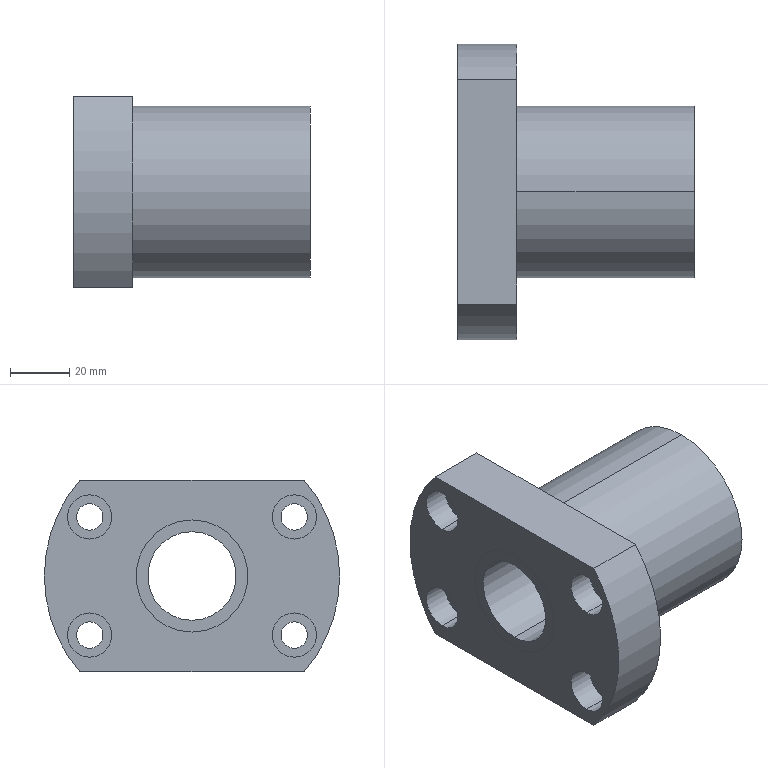Part | SolidWorks | features ICE 3, HoleWzd 1, Revolution 1 | 3 solids | 43 faces | box 80 x 100 x 65 mm | volume 212969 mm3 | cylinder 30 | plane 13 | commonest cylinder face diameters 9 x8 15 x8 38 x6 30 x4 58 x2 100 x2
STEP:
#1=CARTESIAN_POINT('',(9.,34.641,12.5));
#2=VERTEX_POINT('',#1);
#3=CARTESIAN_POINT('',(9.,34.641,27.5));
#4=VERTEX_POINT('',#3);
#5=CARTESIAN_POINT('',(9.,34.641,20.));
#6=DIRECTION('',(-1.,0.,0.));
#7=DIRECTION('',(0.,0.,1.));
#8=AXIS2_PLACEMENT_3D('',#5,#6,#7);
#9=CIRCLE('',#8,7.5);
#10=EDGE_CURVE('',#2,#4,#9,.T.);
#11=ORIENTED_EDGE('',*,*,#10,.F.);
#12=CARTESIAN_POINT('',(0.,34.641,12.5));
#13=VERTEX_POINT('',#12);
#14=CARTESIAN_POINT('',(0.,34.641,12.5));
#15=DIRECTION('',(-1.,0.,0.));
#16=VECTOR('',#15,1000.);
#17=LINE('',#14,#16);
#18=EDGE_CURVE('',#2,#13,#17,.T.);
#19=ORIENTED_EDGE('',*,*,#18,.T.);
#20=CARTESIAN_POINT('',(0.,34.641,27.5));
#21=VERTEX_POINT('',#20);
#22=CARTESIAN_POINT('',(0.,34.641,20.));
#23=DIRECTION('',(-1.,0.,0.));
#24=DIRECTION('',(0.,0.,1.));
#25=AXIS2_PLACEMENT_3D('',#22,#23,#24);
#26=CIRCLE('',#25,7.5);
#27=EDGE_CURVE('',#13,#21,#26,.T.);
#28=ORIENTED_EDGE('',*,*,#27,.T.);
#29=CARTESIAN_POINT('',(0.,34.641,27.5));
#30=DIRECTION('',(-1.,0.,0.));
#31=VECTOR('',#30,1000.);
#32=LINE('',#29,#31);
#33=EDGE_CURVE('',#4,#21,#32,.T.);
#34=ORIENTED_EDGE('',*,*,#33,.F.);
#35=EDGE_LOOP('',(#11,#19,#28,#34));
#36=FACE_OUTER_BOUND('',#35,.T.);
#37=CARTESIAN_POINT('',(0.,34.641,20.));
#38=DIRECTION('',(-1.,0.,0.));
#39=DIRECTION('',(0.,0.,1.));
#40=AXIS2_PLACEMENT_3D('',#37,#38,#39);
#41=CYLINDRICAL_SURFACE('',#40,7.5);
#42=ADVANCED_FACE('',(#36),#41,.F.);
#43=CARTESIAN_POINT('',(20.,34.641,15.5));
#44=VERTEX_POINT('',#43);
#45=CARTESIAN_POINT('',(20.,34.641,24.5));
#46=VERTEX_POINT('',#45);
#47=CARTESIAN_POINT('',(20.,34.641,20.));
#48=DIRECTION('',(-1.,0.,0.));
#49=DIRECTION('',(0.,0.,1.));
#50=AXIS2_PLACEMENT_3D('',#47,#48,#49);
#51=CIRCLE('',#50,4.5);
#52=EDGE_CURVE('',#44,#46,#51,.T.);
#53=ORIENTED_EDGE('',*,*,#52,.F.);
#54=CARTESIAN_POINT('',(9.,34.641,15.5));
#55=VERTEX_POINT('',#54);
#56=CARTESIAN_POINT('',(0.,34.641,15.5));
#57=DIRECTION('',(-1.,0.,0.));
#58=VECTOR('',#57,1000.);
#59=LINE('',#56,#58);
#60=EDGE_CURVE('',#44,#55,#59,.T.);
#61=ORIENTED_EDGE('',*,*,#60,.T.);
#62=CARTESIAN_POINT('',(9.,34.641,24.5));
#63=VERTEX_POINT('',#62);
#64=CARTESIAN_POINT('',(9.,34.641,20.));
#65=DIRECTION('',(-1.,0.,0.));
#66=DIRECTION('',(0.,0.,1.));
#67=AXIS2_PLACEMENT_3D('',#64,#65,#66);
#68=CIRCLE('',#67,4.5);
#69=EDGE_CURVE('',#55,#63,#68,.T.);
#70=ORIENTED_EDGE('',*,*,#69,.T.);
#71=CARTESIAN_POINT('',(0.,34.641,24.5));
#72=DIRECTION('',(-1.,0.,0.));
#73=VECTOR('',#72,1000.);
#74=LINE('',#71,#73);
#75=EDGE_CURVE('',#46,#63,#74,.T.);
#76=ORIENTED_EDGE('',*,*,#75,.F.);
#77=EDGE_LOOP('',(#53,#61,#70,#76));
#78=FACE_OUTER_BOUND('',#77,.T.);
#79=CARTESIAN_POINT('',(0.,34.641,20.));
#80=DIRECTION('',(-1.,0.,0.));
#81=DIRECTION('',(0.,0.,1.));
#82=AXIS2_PLACEMENT_3D('',#79,#80,#81);
#83=CYLINDRICAL_SURFACE('',#82,4.5);
#84=ADVANCED_FACE('',(#78),#83,.F.);
#85=CARTESIAN_POINT('',(9.,34.641,-27.5));
#86=VERTEX_POINT('',#85);
#87=CARTESIAN_POINT('',(9.,34.641,-12.5));
#88=VERTEX_POINT('',#87);
#89=CARTESIAN_POINT('',(9.,34.641,-20.));
#90=DIRECTION('',(-1.,0.,0.));
#91=DIRECTION('',(0.,0.,1.));
#92=AXIS2_PLACEMENT_3D('',#89,#90,#91);
#93=CIRCLE('',#92,7.5);
#94=EDGE_CURVE('',#86,#88,#93,.T.);
#95=ORIENTED_EDGE('',*,*,#94,.F.);
#96=CARTESIAN_POINT('',(0.,34.641,-27.5));
#97=VERTEX_POINT('',#96);
#98=CARTESIAN_POINT('',(0.,34.641,-27.5));
#99=DIRECTION('',(-1.,0.,0.));
#100=VECTOR('',#99,1000.);
#101=LINE('',#98,#100);
#102=EDGE_CURVE('',#86,#97,#101,.T.);
#103=ORIENTED_EDGE('',*,*,#102,.T.);
#104=CARTESIAN_POINT('',(0.,34.641,-12.5));
#105=VERTEX_POINT('',#104);
#106=CARTESIAN_POINT('',(0.,34.641,-20.));
#107=DIRECTION('',(-1.,0.,0.));
#108=DIRECTION('',(0.,0.,1.));
#109=AXIS2_PLACEMENT_3D('',#106,#107,#108);
#110=CIRCLE('',#109,7.5);
#111=EDGE_CURVE('',#97,#105,#110,.T.);
#112=ORIENTED_EDGE('',*,*,#111,.T.);
#113=CARTESIAN_POINT('',(0.,34.641,-12.5));
#114=DIRECTION('',(-1.,0.,0.));
#115=VECTOR('',#114,1000.);
#116=LINE('',#113,#115);
#117=EDGE_CURVE('',#88,#105,#116,.T.);
#118=ORIENTED_EDGE('',*,*,#117,.F.);
#119=EDGE_LOOP('',(#95,#103,#112,#118));
#120=FACE_OUTER_BOUND('',#119,.T.);
#121=CARTESIAN_POINT('',(0.,34.641,-20.));
#122=DIRECTION('',(-1.,0.,0.));
#123=DIRECTION('',(0.,0.,1.));
#124=AXIS2_PLACEMENT_3D('',#121,#122,#123);
#125=CYLINDRICAL_SURFACE('',#124,7.5);
#126=ADVANCED_FACE('',(#120),#125,.F.);
#127=CARTESIAN_POINT('',(20.,34.641,-24.5));
#128=VERTEX_POINT('',#127);
#129=CARTESIAN_POINT('',(20.,34.641,-15.5));
#130=VERTEX_POINT('',#129);
#131=CARTESIAN_POINT('',(20.,34.641,-20.));
#132=DIRECTION('',(-1.,0.,0.));
#133=DIRECTION('',(0.,0.,1.));
#134=AXIS2_PLACEMENT_3D('',#131,#132,#133);
#135=CIRCLE('',#134,4.5);
#136=EDGE_CURVE('',#128,#130,#135,.T.);
#137=ORIENTED_EDGE('',*,*,#136,.F.);
#138=CARTESIAN_POINT('',(9.,34.641,-24.5));
#139=VERTEX_POINT('',#138);
#140=CARTESIAN_POINT('',(0.,34.641,-24.5));
#141=DIRECTION('',(-1.,0.,0.));
#142=VECTOR('',#141,1000.);
#143=LINE('',#140,#142);
#144=EDGE_CURVE('',#128,#139,#143,.T.);
#145=ORIENTED_EDGE('',*,*,#144,.T.);
#146=CARTESIAN_POINT('',(9.,34.641,-15.5));
#147=VERTEX_POINT('',#146);
#148=CARTESIAN_POINT('',(9.,34.641,-20.));
#149=DIRECTION('',(-1.,0.,0.));
#150=DIRECTION('',(0.,0.,1.));
#151=AXIS2_PLACEMENT_3D('',#148,#149,#150);
#152=CIRCLE('',#151,4.5);
#153=EDGE_CURVE('',#139,#147,#152,.T.);
#154=ORIENTED_EDGE('',*,*,#153,.T.);
#155=CARTESIAN_POINT('',(0.,34.641,-15.5));
#156=DIRECTION('',(-1.,0.,0.));
#157=VECTOR('',#156,1000.);
#158=LINE('',#155,#157);
#159=EDGE_CURVE('',#130,#147,#158,.T.);
#160=ORIENTED_EDGE('',*,*,#159,.F.);
#161=EDGE_LOOP('',(#137,#145,#154,#160));
#162=FACE_OUTER_BOUND('',#161,.T.);
#163=CARTESIAN_POINT('',(0.,34.641,-20.));
#164=DIRECTION('',(-1.,0.,0.));
#165=DIRECTION('',(0.,0.,1.));
#166=AXIS2_PLACEMENT_3D('',#163,#164,#165);
#167=CYLINDRICAL_SURFACE('',#166,4.5);
#168=ADVANCED_FACE('',(#162),#167,.F.);
#169=CARTESIAN_POINT('',(9.,-34.641,-27.5));
#170=VERTEX_POINT('',#169);
#171=CARTESIAN_POINT('',(9.,-34.641,-12.5));
#172=VERTEX_POINT('',#171);
#173=CARTESIAN_POINT('',(9.,-34.641,-20.));
#174=DIRECTION('',(-1.,0.,0.));
#175=DIRECTION('',(0.,0.,1.));
#176=AXIS2_PLACEMENT_3D('',#173,#174,#175);
#177=CIRCLE('',#176,7.5);
#178=EDGE_CURVE('',#170,#172,#177,.T.);
#179=ORIENTED_EDGE('',*,*,#178,.F.);
#180=CARTESIAN_POINT('',(0.,-34.641,-27.5));
#181=VERTEX_POINT('',#180);
#182=CARTESIAN_POINT('',(0.,-34.641,-27.5));
#183=DIRECTION('',(-1.,0.,0.));
#184=VECTOR('',#183,1000.);
#185=LINE('',#182,#184);
#186=EDGE_CURVE('',#170,#181,#185,.T.);
#187=ORIENTED_EDGE('',*,*,#186,.T.);
#188=CARTESIAN_POINT('',(0.,-34.641,-12.5));
#189=VERTEX_POINT('',#188);
#190=CARTESIAN_POINT('',(0.,-34.641,-20.));
#191=DIRECTION('',(-1.,0.,0.));
#192=DIRECTION('',(0.,0.,1.));
#193=AXIS2_PLACEMENT_3D('',#190,#191,#192);
#194=CIRCLE('',#193,7.5);
#195=EDGE_CURVE('',#181,#189,#194,.T.);
#196=ORIENTED_EDGE('',*,*,#195,.T.);
#197=CARTESIAN_POINT('',(0.,-34.641,-12.5));
#198=DIRECTION('',(-1.,0.,0.));
#199=VECTOR('',#198,1000.);
#200=LINE('',#197,#199);
#201=EDGE_CURVE('',#172,#189,#200,.T.);
#202=ORIENTED_EDGE('',*,*,#201,.F.);
#203=EDGE_LOOP('',(#179,#187,#196,#202));
#204=FACE_OUTER_BOUND('',#203,.T.);
#205=CARTESIAN_POINT('',(0.,-34.641,-20.));
#206=DIRECTION('',(-1.,0.,0.));
#207=DIRECTION('',(0.,0.,1.));
#208=AXIS2_PLACEMENT_3D('',#205,#206,#207);
#209=CYLINDRICAL_SURFACE('',#208,7.5);
#210=ADVANCED_FACE('',(#204),#209,.F.);
#211=CARTESIAN_POINT('',(20.,-34.641,-24.5));
#212=VERTEX_POINT('',#211);
#213=CARTESIAN_POINT('',(20.,-34.641,-15.5));
#214=VERTEX_POINT('',#213);
#215=CARTESIAN_POINT('',(20.,-34.641,-20.));
#216=DIRECTION('',(-1.,0.,0.));
#217=DIRECTION('',(0.,0.,1.));
#218=AXIS2_PLACEMENT_3D('',#215,#216,#217);
#219=CIRCLE('',#218,4.5);
#220=EDGE_CURVE('',#212,#214,#219,.T.);
#221=ORIENTED_EDGE('',*,*,#220,.F.);
#222=CARTESIAN_POINT('',(9.,-34.641,-24.5));
#223=VERTEX_POINT('',#222);
#224=CARTESIAN_POINT('',(0.,-34.641,-24.5));
#225=DIRECTION('',(-1.,0.,0.));
#226=VECTOR('',#225,1000.);
#227=LINE('',#224,#226);
#228=EDGE_CURVE('',#212,#223,#227,.T.);
#229=ORIENTED_EDGE('',*,*,#228,.T.);
#230=CARTESIAN_POINT('',(9.,-34.641,-15.5));
#231=VERTEX_POINT('',#230);
#232=CARTESIAN_POINT('',(9.,-34.641,-20.));
#233=DIRECTION('',(-1.,0.,0.));
#234=DIRECTION('',(0.,0.,1.));
#235=AXIS2_PLACEMENT_3D('',#232,#233,#234);
#236=CIRCLE('',#235,4.5);
#237=EDGE_CURVE('',#223,#231,#236,.T.);
#238=ORIENTED_EDGE('',*,*,#237,.T.);
#239=CARTESIAN_POINT('',(0.,-34.641,-15.5));
#240=DIRECTION('',(-1.,0.,0.));
#241=VECTOR('',#240,1000.);
#242=LINE('',#239,#241);
#243=EDGE_CURVE('',#214,#231,#242,.T.);
#244=ORIENTED_EDGE('',*,*,#243,.F.);
#245=EDGE_LOOP('',(#221,#229,#238,#244));
#246=FACE_OUTER_BOUND('',#245,.T.);
#247=CARTESIAN_POINT('',(0.,-34.641,-20.));
#248=DIRECTION('',(-1.,0.,0.));
#249=DIRECTION('',(0.,0.,1.));
#250=AXIS2_PLACEMENT_3D('',#247,#248,#249);
#251=CYLINDRICAL_SURFACE('',#250,4.5);
#252=ADVANCED_FACE('',(#246),#251,.F.);
#253=CARTESIAN_POINT('',(9.,-34.641,12.5));
#254=VERTEX_POINT('',#253);
#255=CARTESIAN_POINT('',(9.,-34.641,27.5));
#256=VERTEX_POINT('',#255);
#257=CARTESIAN_POINT('',(9.,-34.641,20.));
#258=DIRECTION('',(-1.,0.,0.));
#259=DIRECTION('',(0.,0.,1.));
#260=AXIS2_PLACEMENT_3D('',#257,#258,#259);
#261=CIRCLE('',#260,7.5);
#262=EDGE_CURVE('',#254,#256,#261,.T.);
#263=ORIENTED_EDGE('',*,*,#262,.F.);
#264=CARTESIAN_POINT('',(0.,-34.641,12.5));
#265=VERTEX_POINT('',#264);
#266=CARTESIAN_POINT('',(0.,-34.641,12.5));
#267=DIRECTION('',(-1.,0.,0.));
#268=VECTOR('',#267,1000.);
#269=LINE('',#266,#268);
#270=EDGE_CURVE('',#254,#265,#269,.T.);
#271=ORIENTED_EDGE('',*,*,#270,.T.);
#272=CARTESIAN_POINT('',(0.,-34.641,27.5));
#273=VERTEX_POINT('',#272);
#274=CARTESIAN_POINT('',(0.,-34.641,20.));
#275=DIRECTION('',(-1.,0.,0.));
#276=DIRECTION('',(0.,0.,1.));
#277=AXIS2_PLACEMENT_3D('',#274,#275,#276);
#278=CIRCLE('',#277,7.5);
#279=EDGE_CURVE('',#265,#273,#278,.T.);
#280=ORIENTED_EDGE('',*,*,#279,.T.);
#281=CARTESIAN_POINT('',(0.,-34.641,27.5));
#282=DIRECTION('',(-1.,0.,0.));
#283=VECTOR('',#282,1000.);
#284=LINE('',#281,#283);
#285=EDGE_CURVE('',#256,#273,#284,.T.);
#286=ORIENTED_EDGE('',*,*,#285,.F.);
#287=EDGE_LOOP('',(#263,#271,#280,#286));
#288=FACE_OUTER_BOUND('',#287,.T.);
#289=CARTESIAN_POINT('',(0.,-34.641,20.));
#290=DIRECTION('',(-1.,0.,0.));
#291=DIRECTION('',(0.,0.,1.));
#292=AXIS2_PLACEMENT_3D('',#289,#290,#291);
#293=CYLINDRICAL_SURFACE('',#292,7.5);
#294=ADVANCED_FACE('',(#288),#293,.F.);
#295=CARTESIAN_POINT('',(20.,-34.641,15.5));
#296=VERTEX_POINT('',#295);
#297=CARTESIAN_POINT('',(20.,-34.641,24.5));
#298=VERTEX_POINT('',#297);
#299=CARTESIAN_POINT('',(20.,-34.641,20.));
#300=DIRECTION('',(-1.,0.,0.));
#301=DIRECTION('',(0.,0.,1.));
#302=AXIS2_PLACEMENT_3D('',#299,#300,#301);
#303=CIRCLE('',#302,4.5);
#304=EDGE_CURVE('',#296,#298,#303,.T.);
#305=ORIENTED_EDGE('',*,*,#304,.F.);
#306=CARTESIAN_POINT('',(9.,-34.641,15.5));
#307=VERTEX_POINT('',#306);
#308=CARTESIAN_POINT('',(0.,-34.641,15.5));
#309=DIRECTION('',(-1.,0.,0.));
#310=VECTOR('',#309,1000.);
#311=LINE('',#308,#310);
#312=EDGE_CURVE('',#296,#307,#311,.T.);
#313=ORIENTED_EDGE('',*,*,#312,.T.);
#314=CARTESIAN_POINT('',(9.,-34.641,24.5));
#315=VERTEX_POINT('',#314);
#316=CARTESIAN_POINT('',(9.,-34.641,20.));
#317=DIRECTION('',(-1.,0.,0.));
#318=DIRECTION('',(0.,0.,1.));
#319=AXIS2_PLACEMENT_3D('',#316,#317,#318);
#320=CIRCLE('',#319,4.5);
#321=EDGE_CURVE('',#307,#315,#320,.T.);
#322=ORIENTED_EDGE('',*,*,#321,.T.);
#323=CARTESIAN_POINT('',(0.,-34.641,24.5));
#324=DIRECTION('',(-1.,0.,0.));
#325=VECTOR('',#324,1000.);
#326=LINE('',#323,#325);
#327=EDGE_CURVE('',#298,#315,#326,.T.);
#328=ORIENTED_EDGE('',*,*,#327,.F.);
#329=EDGE_LOOP('',(#305,#313,#322,#328));
#330=FACE_OUTER_BOUND('',#329,.T.);
#331=CARTESIAN_POINT('',(0.,-34.641,20.));
#332=DIRECTION('',(-1.,0.,0.));
#333=DIRECTION('',(0.,0.,1.));
#334=AXIS2_PLACEMENT_3D('',#331,#332,#333);
#335=CYLINDRICAL_SURFACE('',#334,4.5);
#336=ADVANCED_FACE('',(#330),#335,.F.);
#337=CARTESIAN_POINT('',(80.,0.,-19.));
#338=VERTEX_POINT('',#337);
#339=CARTESIAN_POINT('',(80.,0.,19.));
#340=VERTEX_POINT('',#339);
#341=CARTESIAN_POINT('',(80.,0.,0.));
#342=DIRECTION('',(-1.,0.,0.));
#343=DIRECTION('',(0.,0.,1.));
#344=AXIS2_PLACEMENT_3D('',#341,#342,#343);
#345=CIRCLE('',#344,19.);
#346=EDGE_CURVE('',#338,#340,#345,.T.);
#347=ORIENTED_EDGE('',*,*,#346,.F.);
#348=CARTESIAN_POINT('',(0.,0.,-19.));
#349=VERTEX_POINT('',#348);
#350=CARTESIAN_POINT('',(0.,0.,-19.));
#351=DIRECTION('',(-1.,0.,0.));
#352=VECTOR('',#351,1000.);
#353=LINE('',#350,#352);
#354=EDGE_CURVE('',#338,#349,#353,.T.);
#355=ORIENTED_EDGE('',*,*,#354,.T.);
#356=CARTESIAN_POINT('',(0.,0.,19.));
#357=VERTEX_POINT('',#356);
#358=CARTESIAN_POINT('',(0.,0.,0.));
#359=DIRECTION('',(-1.,0.,0.));
#360=DIRECTION('',(0.,0.,1.));
#361=AXIS2_PLACEMENT_3D('',#358,#359,#360);
#362=CIRCLE('',#361,19.);
#363=EDGE_CURVE('',#349,#357,#362,.T.);
#364=ORIENTED_EDGE('',*,*,#363,.T.);
#365=CARTESIAN_POINT('',(0.,0.,19.));
#366=DIRECTION('',(-1.,0.,0.));
#367=VECTOR('',#366,1000.);
#368=LINE('',#365,#367);
#369=EDGE_CURVE('',#340,#357,#368,.T.);
#370=ORIENTED_EDGE('',*,*,#369,.F.);
#371=EDGE_LOOP('',(#347,#355,#364,#370));
#372=FACE_OUTER_BOUND('',#371,.T.);
#373=CARTESIAN_POINT('',(0.,0.,0.));
#374=DIRECTION('',(-1.,0.,0.));
#375=DIRECTION('',(0.,0.,1.));
#376=AXIS2_PLACEMENT_3D('',#373,#374,#375);
#377=CYLINDRICAL_SURFACE('',#376,19.);
#378=ADVANCED_FACE('',(#372),#377,.F.);
#379=CARTESIAN_POINT('',(80.,0.,29.));
#380=VERTEX_POINT('',#379);
#381=CARTESIAN_POINT('',(80.,0.,-29.));
#382=VERTEX_POINT('',#381);
#383=CARTESIAN_POINT('',(80.,0.,0.));
#384=DIRECTION('',(-1.,0.,0.));
#385=DIRECTION('',(0.,0.,1.));
#386=AXIS2_PLACEMENT_3D('',#383,#384,#385);
#387=CIRCLE('',#386,29.);
#388=EDGE_CURVE('',#380,#382,#387,.T.);
#389=ORIENTED_EDGE('',*,*,#388,.T.);
#390=CARTESIAN_POINT('',(20.,0.,-29.));
#391=VERTEX_POINT('',#390);
#392=CARTESIAN_POINT('',(0.,0.,-29.));
#393=DIRECTION('',(-1.,0.,0.));
#394=VECTOR('',#393,1000.);
#395=LINE('',#392,#394);
#396=EDGE_CURVE('',#382,#391,#395,.T.);
#397=ORIENTED_EDGE('',*,*,#396,.T.);
#398=CARTESIAN_POINT('',(20.,0.,29.));
#399=VERTEX_POINT('',#398);
#400=CARTESIAN_POINT('',(20.,0.,0.));
#401=DIRECTION('',(-1.,0.,0.));
#402=DIRECTION('',(0.,0.,1.));
#403=AXIS2_PLACEMENT_3D('',#400,#401,#402);
#404=CIRCLE('',#403,29.);
#405=EDGE_CURVE('',#399,#391,#404,.T.);
#406=ORIENTED_EDGE('',*,*,#405,.F.);
#407=CARTESIAN_POINT('',(0.,0.,29.));
#408=DIRECTION('',(-1.,0.,0.));
#409=VECTOR('',#408,1000.);
#410=LINE('',#407,#409);
#411=EDGE_CURVE('',#380,#399,#410,.T.);
#412=ORIENTED_EDGE('',*,*,#411,.F.);
#413=EDGE_LOOP('',(#389,#397,#406,#412));
#414=FACE_OUTER_BOUND('',#413,.T.);
#415=CARTESIAN_POINT('',(0.,0.,0.));
#416=DIRECTION('',(-1.,0.,0.));
#417=DIRECTION('',(0.,0.,1.));
#418=AXIS2_PLACEMENT_3D('',#415,#416,#417);
#419=CYLINDRICAL_SURFACE('',#418,29.);
#420=ADVANCED_FACE('',(#414),#419,.T.);
#421=CARTESIAN_POINT('',(20.,37.997,32.5));
#422=VERTEX_POINT('',#421);
#423=CARTESIAN_POINT('',(0.,37.997,32.5));
#424=VERTEX_POINT('',#423);
#425=CARTESIAN_POINT('',(0.,37.997,32.5));
#426=DIRECTION('',(-1.,0.,0.));
#427=VECTOR('',#426,1000.);
#428=LINE('',#425,#427);
#429=EDGE_CURVE('',#422,#424,#428,.T.);
#430=ORIENTED_EDGE('',*,*,#429,.F.);
#431=CARTESIAN_POINT('',(20.,37.997,-32.5));
#432=VERTEX_POINT('',#431);
#433=CARTESIAN_POINT('',(20.,0.,0.));
#434=DIRECTION('',(-1.,0.,0.));
#435=DIRECTION('',(0.,0.,1.));
#436=AXIS2_PLACEMENT_3D('',#433,#434,#435);
#437=CIRCLE('',#436,50.);
#438=EDGE_CURVE('',#422,#432,#437,.T.);
#439=ORIENTED_EDGE('',*,*,#438,.T.);
#440=CARTESIAN_POINT('',(0.,37.997,-32.5));
#441=VERTEX_POINT('',#440);
#442=CARTESIAN_POINT('',(0.,37.997,-32.5));
#443=DIRECTION('',(1.,0.,0.));
#444=VECTOR('',#443,1000.);
#445=LINE('',#442,#444);
#446=EDGE_CURVE('',#441,#432,#445,.T.);
#447=ORIENTED_EDGE('',*,*,#446,.F.);
#448=CARTESIAN_POINT('',(0.,0.,0.));
#449=DIRECTION('',(-1.,0.,0.));
#450=DIRECTION('',(0.,0.,1.));
#451=AXIS2_PLACEMENT_3D('',#448,#449,#450);
#452=CIRCLE('',#451,50.);
#453=EDGE_CURVE('',#424,#441,#452,.T.);
#454=ORIENTED_EDGE('',*,*,#453,.F.);
#455=EDGE_LOOP('',(#430,#439,#447,#454));
#456=FACE_OUTER_BOUND('',#455,.T.);
#457=CARTESIAN_POINT('',(0.,0.,0.));
#458=DIRECTION('',(-1.,0.,0.));
#459=DIRECTION('',(0.,0.,1.));
#460=AXIS2_PLACEMENT_3D('',#457,#458,#459);
#461=CYLINDRICAL_SURFACE('',#460,50.);
#462=ADVANCED_FACE('',(#456),#461,.T.);
#463=CARTESIAN_POINT('',(0.,-37.997,32.5));
#464=VERTEX_POINT('',#463);
#465=CARTESIAN_POINT('',(20.,-37.997,32.5));
#466=VERTEX_POINT('',#465);
#467=CARTESIAN_POINT('',(0.,-37.997,32.5));
#468=DIRECTION('',(1.,0.,0.));
#469=VECTOR('',#468,1000.);
#470=LINE('',#467,#469);
#471=EDGE_CURVE('',#464,#466,#470,.T.);
#472=ORIENTED_EDGE('',*,*,#471,.F.);
#473=CARTESIAN_POINT('',(0.,-37.997,-32.5));
#474=VERTEX_POINT('',#473);
#475=CARTESIAN_POINT('',(0.,0.,0.));
#476=DIRECTION('',(-1.,0.,0.));
#477=DIRECTION('',(0.,0.,1.));
#478=AXIS2_PLACEMENT_3D('',#475,#476,#477);
#479=CIRCLE('',#478,50.);
#480=EDGE_CURVE('',#474,#464,#479,.T.);
#481=ORIENTED_EDGE('',*,*,#480,.F.);
#482=CARTESIAN_POINT('',(20.,-37.997,-32.5));
#483=VERTEX_POINT('',#482);
#484=CARTESIAN_POINT('',(0.,-37.997,-32.5));
#485=DIRECTION('',(-1.,0.,0.));
#486=VECTOR('',#485,1000.);
#487=LINE('',#484,#486);
#488=EDGE_CURVE('',#483,#474,#487,.T.);
#489=ORIENTED_EDGE('',*,*,#488,.F.);
#490=CARTESIAN_POINT('',(20.,0.,0.));
#491=DIRECTION('',(-1.,0.,0.));
#492=DIRECTION('',(0.,0.,1.));
#493=AXIS2_PLACEMENT_3D('',#490,#491,#492);
#494=CIRCLE('',#493,50.);
#495=EDGE_CURVE('',#483,#466,#494,.T.);
#496=ORIENTED_EDGE('',*,*,#495,.T.);
#497=EDGE_LOOP('',(#472,#481,#489,#496));
#498=FACE_OUTER_BOUND('',#497,.T.);
#499=CARTESIAN_POINT('',(0.,0.,0.));
#500=DIRECTION('',(-1.,0.,0.));
#501=DIRECTION('',(0.,0.,1.));
#502=AXIS2_PLACEMENT_3D('',#499,#500,#501);
#503=CYLINDRICAL_SURFACE('',#502,50.);
#504=ADVANCED_FACE('',(#498),#503,.T.);
#505=CARTESIAN_POINT('',(20.,34.641,20.));
#506=DIRECTION('',(-1.,0.,0.));
#507=DIRECTION('',(0.,0.,1.));
#508=AXIS2_PLACEMENT_3D('',#505,#506,#507);
#509=CIRCLE('',#508,4.5);
#510=EDGE_CURVE('',#46,#44,#509,.T.);
#511=ORIENTED_EDGE('',*,*,#510,.T.);
#512=ORIENTED_EDGE('',*,*,#52,.T.);
#513=EDGE_LOOP('',(#511,#512));
#514=FACE_BOUND('',#513,.T.);
#515=CARTESIAN_POINT('',(20.,34.641,-20.));
#516=DIRECTION('',(-1.,0.,0.));
#517=DIRECTION('',(0.,0.,1.));
#518=AXIS2_PLACEMENT_3D('',#515,#516,#517);
#519=CIRCLE('',#518,4.5);
#520=EDGE_CURVE('',#130,#128,#519,.T.);
#521=ORIENTED_EDGE('',*,*,#520,.T.);
#522=ORIENTED_EDGE('',*,*,#136,.T.);
#523=EDGE_LOOP('',(#521,#522));
#524=FACE_BOUND('',#523,.T.);
#525=CARTESIAN_POINT('',(20.,-34.641,-20.));
#526=DIRECTION('',(-1.,0.,0.));
#527=DIRECTION('',(0.,0.,1.));
#528=AXIS2_PLACEMENT_3D('',#525,#526,#527);
#529=CIRCLE('',#528,4.5);
#530=EDGE_CURVE('',#214,#212,#529,.T.);
#531=ORIENTED_EDGE('',*,*,#530,.T.);
#532=ORIENTED_EDGE('',*,*,#220,.T.);
#533=EDGE_LOOP('',(#531,#532));
#534=FACE_BOUND('',#533,.T.);
#535=CARTESIAN_POINT('',(20.,-34.641,20.));
#536=DIRECTION('',(-1.,0.,0.));
#537=DIRECTION('',(0.,0.,1.));
#538=AXIS2_PLACEMENT_3D('',#535,#536,#537);
#539=CIRCLE('',#538,4.5);
#540=EDGE_CURVE('',#298,#296,#539,.T.);
#541=ORIENTED_EDGE('',*,*,#540,.T.);
#542=ORIENTED_EDGE('',*,*,#304,.T.);
#543=EDGE_LOOP('',(#541,#542));
#544=FACE_BOUND('',#543,.T.);
#545=ORIENTED_EDGE('',*,*,#405,.T.);
#546=CARTESIAN_POINT('',(20.,0.,0.));
#547=DIRECTION('',(-1.,0.,0.));
#548=DIRECTION('',(0.,0.,1.));
#549=AXIS2_PLACEMENT_3D('',#546,#547,#548);
#550=CIRCLE('',#549,29.);
#551=EDGE_CURVE('',#391,#399,#550,.T.);
#552=ORIENTED_EDGE('',*,*,#551,.T.);
#553=EDGE_LOOP('',(#545,#552));
#554=FACE_BOUND('',#553,.T.);
#555=CARTESIAN_POINT('',(20.,50.,32.5));
#556=DIRECTION('',(0.,1.,0.));
#557=VECTOR('',#556,1000.);
#558=LINE('',#555,#557);
#559=EDGE_CURVE('',#466,#422,#558,.T.);
#560=ORIENTED_EDGE('',*,*,#559,.F.);
#561=ORIENTED_EDGE('',*,*,#495,.F.);
#562=CARTESIAN_POINT('',(20.,50.,-32.5));
#563=DIRECTION('',(0.,-1.,0.));
#564=VECTOR('',#563,1000.);
#565=LINE('',#562,#564);
#566=EDGE_CURVE('',#432,#483,#565,.T.);
#567=ORIENTED_EDGE('',*,*,#566,.F.);
#568=ORIENTED_EDGE('',*,*,#438,.F.);
#569=EDGE_LOOP('',(#560,#561,#567,#568));
#570=FACE_OUTER_BOUND('',#569,.T.);
#571=CARTESIAN_POINT('',(20.,50.,0.));
#572=DIRECTION('',(-1.,0.,0.));
#573=DIRECTION('',(0.,0.,1.));
#574=AXIS2_PLACEMENT_3D('',#571,#572,#573);
#575=PLANE('',#574);
#576=ADVANCED_FACE('',(#514,#524,#534,#544,#554,#570),#575,.F.);
#577=CARTESIAN_POINT('',(0.,34.641,20.));
#578=DIRECTION('',(-1.,0.,0.));
#579=DIRECTION('',(0.,0.,1.));
#580=AXIS2_PLACEMENT_3D('',#577,#578,#579);
#581=CIRCLE('',#580,7.5);
#582=EDGE_CURVE('',#21,#13,#581,.T.);
#583=ORIENTED_EDGE('',*,*,#582,.F.);
#584=ORIENTED_EDGE('',*,*,#27,.F.);
#585=EDGE_LOOP('',(#583,#584));
#586=FACE_BOUND('',#585,.T.);
#587=CARTESIAN_POINT('',(0.,34.641,-20.));
#588=DIRECTION('',(-1.,0.,0.));
#589=DIRECTION('',(0.,0.,1.));
#590=AXIS2_PLACEMENT_3D('',#587,#588,#589);
#591=CIRCLE('',#590,7.5);
#592=EDGE_CURVE('',#105,#97,#591,.T.);
#593=ORIENTED_EDGE('',*,*,#592,.F.);
#594=ORIENTED_EDGE('',*,*,#111,.F.);
#595=EDGE_LOOP('',(#593,#594));
#596=FACE_BOUND('',#595,.T.);
#597=CARTESIAN_POINT('',(0.,-34.641,-20.));
#598=DIRECTION('',(-1.,0.,0.));
#599=DIRECTION('',(0.,0.,1.));
#600=AXIS2_PLACEMENT_3D('',#597,#598,#599);
#601=CIRCLE('',#600,7.5);
#602=EDGE_CURVE('',#189,#181,#601,.T.);
#603=ORIENTED_EDGE('',*,*,#602,.F.);
#604=ORIENTED_EDGE('',*,*,#195,.F.);
#605=EDGE_LOOP('',(#603,#604));
#606=FACE_BOUND('',#605,.T.);
#607=CARTESIAN_POINT('',(0.,-34.641,20.));
#608=DIRECTION('',(-1.,0.,0.));
#609=DIRECTION('',(0.,0.,1.));
#610=AXIS2_PLACEMENT_3D('',#607,#608,#609);
#611=CIRCLE('',#610,7.5);
#612=EDGE_CURVE('',#273,#265,#611,.T.);
#613=ORIENTED_EDGE('',*,*,#612,.F.);
#614=ORIENTED_EDGE('',*,*,#279,.F.);
#615=EDGE_LOOP('',(#613,#614));
#616=FACE_BOUND('',#615,.T.);
#617=CARTESIAN_POINT('',(0.,0.,0.));
#618=DIRECTION('',(-1.,0.,0.));
#619=DIRECTION('',(0.,0.,1.));
#620=AXIS2_PLACEMENT_3D('',#617,#618,#619);
#621=CIRCLE('',#620,19.);
#622=EDGE_CURVE('',#357,#349,#621,.T.);
#623=ORIENTED_EDGE('',*,*,#622,.F.);
#624=ORIENTED_EDGE('',*,*,#363,.F.);
#625=EDGE_LOOP('',(#623,#624));
#626=FACE_BOUND('',#625,.T.);
#627=CARTESIAN_POINT('',(0.,19.,32.5));
#628=DIRECTION('',(0.,-1.,0.));
#629=VECTOR('',#628,1000.);
#630=LINE('',#627,#629);
#631=EDGE_CURVE('',#424,#464,#630,.T.);
#632=ORIENTED_EDGE('',*,*,#631,.F.);
#633=ORIENTED_EDGE('',*,*,#453,.T.);
#634=CARTESIAN_POINT('',(0.,19.,-32.5));
#635=DIRECTION('',(0.,1.,0.));
#636=VECTOR('',#635,1000.);
#637=LINE('',#634,#636);
#638=EDGE_CURVE('',#474,#441,#637,.T.);
#639=ORIENTED_EDGE('',*,*,#638,.F.);
#640=ORIENTED_EDGE('',*,*,#480,.T.);
#641=EDGE_LOOP('',(#632,#633,#639,#640));
#642=FACE_OUTER_BOUND('',#641,.T.);
#643=CARTESIAN_POINT('',(0.,19.,0.));
#644=DIRECTION('',(1.,0.,0.));
#645=DIRECTION('',(0.,0.,-1.));
#646=AXIS2_PLACEMENT_3D('',#643,#644,#645);
#647=PLANE('',#646);
#648=ADVANCED_FACE('',(#586,#596,#606,#616,#626,#642),#647,.F.);
#649=ORIENTED_EDGE('',*,*,#396,.F.);
#650=CARTESIAN_POINT('',(80.,0.,0.));
#651=DIRECTION('',(-1.,0.,0.));
#652=DIRECTION('',(0.,0.,1.));
#653=AXIS2_PLACEMENT_3D('',#650,#651,#652);
#654=CIRCLE('',#653,29.);
#655=EDGE_CURVE('',#382,#380,#654,.T.);
#656=ORIENTED_EDGE('',*,*,#655,.T.);
#657=ORIENTED_EDGE('',*,*,#411,.T.);
#658=ORIENTED_EDGE('',*,*,#551,.F.);
#659=EDGE_LOOP('',(#649,#656,#657,#658));
#660=FACE_OUTER_BOUND('',#659,.T.);
#661=CARTESIAN_POINT('',(0.,0.,0.));
#662=DIRECTION('',(-1.,0.,0.));
#663=DIRECTION('',(0.,0.,1.));
#664=AXIS2_PLACEMENT_3D('',#661,#662,#663);
#665=CYLINDRICAL_SURFACE('',#664,29.);
#666=ADVANCED_FACE('',(#660),#665,.T.);
#667=ORIENTED_EDGE('',*,*,#388,.F.);
#668=ORIENTED_EDGE('',*,*,#655,.F.);
#669=EDGE_LOOP('',(#667,#668));
#670=FACE_OUTER_BOUND('',#669,.T.);
#671=CARTESIAN_POINT('',(80.,0.,0.));
#672=DIRECTION('',(-1.,0.,0.));
#673=DIRECTION('',(0.,0.,1.));
#674=AXIS2_PLACEMENT_3D('',#671,#672,#673);
#675=CIRCLE('',#674,19.);
#676=EDGE_CURVE('',#340,#338,#675,.T.);
#677=ORIENTED_EDGE('',*,*,#676,.T.);
#678=ORIENTED_EDGE('',*,*,#346,.T.);
#679=EDGE_LOOP('',(#677,#678));
#680=FACE_BOUND('',#679,.T.);
#681=CARTESIAN_POINT('',(80.,29.,0.));
#682=DIRECTION('',(-1.,0.,0.));
#683=DIRECTION('',(0.,0.,1.));
#684=AXIS2_PLACEMENT_3D('',#681,#682,#683);
#685=PLANE('',#684);
#686=ADVANCED_FACE('',(#670,#680),#685,.F.);
#687=ORIENTED_EDGE('',*,*,#354,.F.);
#688=ORIENTED_EDGE('',*,*,#676,.F.);
#689=ORIENTED_EDGE('',*,*,#369,.T.);
#690=ORIENTED_EDGE('',*,*,#622,.T.);
#691=EDGE_LOOP('',(#687,#688,#689,#690));
#692=FACE_OUTER_BOUND('',#691,.T.);
#693=CARTESIAN_POINT('',(0.,0.,0.));
#694=DIRECTION('',(-1.,0.,0.));
#695=DIRECTION('',(0.,0.,1.));
#696=AXIS2_PLACEMENT_3D('',#693,#694,#695);
#697=CYLINDRICAL_SURFACE('',#696,19.);
#698=ADVANCED_FACE('',(#692),#697,.F.);
#699=ORIENTED_EDGE('',*,*,#312,.F.);
#700=ORIENTED_EDGE('',*,*,#540,.F.);
#701=ORIENTED_EDGE('',*,*,#327,.T.);
#702=CARTESIAN_POINT('',(9.,-34.641,20.));
#703=DIRECTION('',(-1.,0.,0.));
#704=DIRECTION('',(0.,0.,1.));
#705=AXIS2_PLACEMENT_3D('',#702,#703,#704);
#706=CIRCLE('',#705,4.5);
#707=EDGE_CURVE('',#315,#307,#706,.T.);
#708=ORIENTED_EDGE('',*,*,#707,.T.);
#709=EDGE_LOOP('',(#699,#700,#701,#708));
#710=FACE_OUTER_BOUND('',#709,.T.);
#711=CARTESIAN_POINT('',(0.,-34.641,20.));
#712=DIRECTION('',(-1.,0.,0.));
#713=DIRECTION('',(0.,0.,1.));
#714=AXIS2_PLACEMENT_3D('',#711,#712,#713);
#715=CYLINDRICAL_SURFACE('',#714,4.5);
#716=ADVANCED_FACE('',(#710),#715,.F.);
#717=ORIENTED_EDGE('',*,*,#707,.F.);
#718=ORIENTED_EDGE('',*,*,#321,.F.);
#719=EDGE_LOOP('',(#717,#718));
#720=FACE_BOUND('',#719,.T.);
#721=CARTESIAN_POINT('',(9.,-34.641,20.));
#722=DIRECTION('',(-1.,0.,0.));
#723=DIRECTION('',(0.,0.,1.));
#724=AXIS2_PLACEMENT_3D('',#721,#722,#723);
#725=CIRCLE('',#724,7.5);
#726=EDGE_CURVE('',#256,#254,#725,.T.);
#727=ORIENTED_EDGE('',*,*,#726,.T.);
#728=ORIENTED_EDGE('',*,*,#262,.T.);
#729=EDGE_LOOP('',(#727,#728));
#730=FACE_OUTER_BOUND('',#729,.T.);
#731=CARTESIAN_POINT('',(9.,-30.141,20.));
#732=DIRECTION('',(1.,0.,0.));
#733=DIRECTION('',(0.,0.,-1.));
#734=AXIS2_PLACEMENT_3D('',#731,#732,#733);
#735=PLANE('',#734);
#736=ADVANCED_FACE('',(#720,#730),#735,.F.);
#737=ORIENTED_EDGE('',*,*,#270,.F.);
#738=ORIENTED_EDGE('',*,*,#726,.F.);
#739=ORIENTED_EDGE('',*,*,#285,.T.);
#740=ORIENTED_EDGE('',*,*,#612,.T.);
#741=EDGE_LOOP('',(#737,#738,#739,#740));
#742=FACE_OUTER_BOUND('',#741,.T.);
#743=CARTESIAN_POINT('',(0.,-34.641,20.));
#744=DIRECTION('',(-1.,0.,0.));
#745=DIRECTION('',(0.,0.,1.));
#746=AXIS2_PLACEMENT_3D('',#743,#744,#745);
#747=CYLINDRICAL_SURFACE('',#746,7.5);
#748=ADVANCED_FACE('',(#742),#747,.F.);
#749=ORIENTED_EDGE('',*,*,#228,.F.);
#750=ORIENTED_EDGE('',*,*,#530,.F.);
#751=ORIENTED_EDGE('',*,*,#243,.T.);
#752=CARTESIAN_POINT('',(9.,-34.641,-20.));
#753=DIRECTION('',(-1.,0.,0.));
#754=DIRECTION('',(0.,0.,1.));
#755=AXIS2_PLACEMENT_3D('',#752,#753,#754);
#756=CIRCLE('',#755,4.5);
#757=EDGE_CURVE('',#231,#223,#756,.T.);
#758=ORIENTED_EDGE('',*,*,#757,.T.);
#759=EDGE_LOOP('',(#749,#750,#751,#758));
#760=FACE_OUTER_BOUND('',#759,.T.);
#761=CARTESIAN_POINT('',(0.,-34.641,-20.));
#762=DIRECTION('',(-1.,0.,0.));
#763=DIRECTION('',(0.,0.,1.));
#764=AXIS2_PLACEMENT_3D('',#761,#762,#763);
#765=CYLINDRICAL_SURFACE('',#764,4.5);
#766=ADVANCED_FACE('',(#760),#765,.F.);
#767=ORIENTED_EDGE('',*,*,#757,.F.);
#768=ORIENTED_EDGE('',*,*,#237,.F.);
#769=EDGE_LOOP('',(#767,#768));
#770=FACE_BOUND('',#769,.T.);
#771=CARTESIAN_POINT('',(9.,-34.641,-20.));
#772=DIRECTION('',(-1.,0.,0.));
#773=DIRECTION('',(0.,0.,1.));
#774=AXIS2_PLACEMENT_3D('',#771,#772,#773);
#775=CIRCLE('',#774,7.5);
#776=EDGE_CURVE('',#172,#170,#775,.T.);
#777=ORIENTED_EDGE('',*,*,#776,.T.);
#778=ORIENTED_EDGE('',*,*,#178,.T.);
#779=EDGE_LOOP('',(#777,#778));
#780=FACE_OUTER_BOUND('',#779,.T.);
#781=CARTESIAN_POINT('',(9.,-30.141,-20.));
#782=DIRECTION('',(1.,0.,0.));
#783=DIRECTION('',(0.,0.,-1.));
#784=AXIS2_PLACEMENT_3D('',#781,#782,#783);
#785=PLANE('',#784);
#786=ADVANCED_FACE('',(#770,#780),#785,.F.);
#787=ORIENTED_EDGE('',*,*,#186,.F.);
#788=ORIENTED_EDGE('',*,*,#776,.F.);
#789=ORIENTED_EDGE('',*,*,#201,.T.);
#790=ORIENTED_EDGE('',*,*,#602,.T.);
#791=EDGE_LOOP('',(#787,#788,#789,#790));
#792=FACE_OUTER_BOUND('',#791,.T.);
#793=CARTESIAN_POINT('',(0.,-34.641,-20.));
#794=DIRECTION('',(-1.,0.,0.));
#795=DIRECTION('',(0.,0.,1.));
#796=AXIS2_PLACEMENT_3D('',#793,#794,#795);
#797=CYLINDRICAL_SURFACE('',#796,7.5);
#798=ADVANCED_FACE('',(#792),#797,.F.);
#799=ORIENTED_EDGE('',*,*,#144,.F.);
#800=ORIENTED_EDGE('',*,*,#520,.F.);
#801=ORIENTED_EDGE('',*,*,#159,.T.);
#802=CARTESIAN_POINT('',(9.,34.641,-20.));
#803=DIRECTION('',(-1.,0.,0.));
#804=DIRECTION('',(0.,0.,1.));
#805=AXIS2_PLACEMENT_3D('',#802,#803,#804);
#806=CIRCLE('',#805,4.5);
#807=EDGE_CURVE('',#147,#139,#806,.T.);
#808=ORIENTED_EDGE('',*,*,#807,.T.);
#809=EDGE_LOOP('',(#799,#800,#801,#808));
#810=FACE_OUTER_BOUND('',#809,.T.);
#811=CARTESIAN_POINT('',(0.,34.641,-20.));
#812=DIRECTION('',(-1.,0.,0.));
#813=DIRECTION('',(0.,0.,1.));
#814=AXIS2_PLACEMENT_3D('',#811,#812,#813);
#815=CYLINDRICAL_SURFACE('',#814,4.5);
#816=ADVANCED_FACE('',(#810),#815,.F.);
#817=ORIENTED_EDGE('',*,*,#807,.F.);
#818=ORIENTED_EDGE('',*,*,#153,.F.);
#819=EDGE_LOOP('',(#817,#818));
#820=FACE_BOUND('',#819,.T.);
#821=CARTESIAN_POINT('',(9.,34.641,-20.));
#822=DIRECTION('',(-1.,0.,0.));
#823=DIRECTION('',(0.,0.,1.));
#824=AXIS2_PLACEMENT_3D('',#821,#822,#823);
#825=CIRCLE('',#824,7.5);
#826=EDGE_CURVE('',#88,#86,#825,.T.);
#827=ORIENTED_EDGE('',*,*,#826,.T.);
#828=ORIENTED_EDGE('',*,*,#94,.T.);
#829=EDGE_LOOP('',(#827,#828));
#830=FACE_OUTER_BOUND('',#829,.T.);
#831=CARTESIAN_POINT('',(9.,39.141,-20.));
#832=DIRECTION('',(1.,0.,0.));
#833=DIRECTION('',(0.,0.,-1.));
#834=AXIS2_PLACEMENT_3D('',#831,#832,#833);
#835=PLANE('',#834);
#836=ADVANCED_FACE('',(#820,#830),#835,.F.);
#837=ORIENTED_EDGE('',*,*,#102,.F.);
#838=ORIENTED_EDGE('',*,*,#826,.F.);
#839=ORIENTED_EDGE('',*,*,#117,.T.);
#840=ORIENTED_EDGE('',*,*,#592,.T.);
#841=EDGE_LOOP('',(#837,#838,#839,#840));
#842=FACE_OUTER_BOUND('',#841,.T.);
#843=CARTESIAN_POINT('',(0.,34.641,-20.));
#844=DIRECTION('',(-1.,0.,0.));
#845=DIRECTION('',(0.,0.,1.));
#846=AXIS2_PLACEMENT_3D('',#843,#844,#845);
#847=CYLINDRICAL_SURFACE('',#846,7.5);
#848=ADVANCED_FACE('',(#842),#847,.F.);
#849=ORIENTED_EDGE('',*,*,#60,.F.);
#850=ORIENTED_EDGE('',*,*,#510,.F.);
#851=ORIENTED_EDGE('',*,*,#75,.T.);
#852=CARTESIAN_POINT('',(9.,34.641,20.));
#853=DIRECTION('',(-1.,0.,0.));
#854=DIRECTION('',(0.,0.,1.));
#855=AXIS2_PLACEMENT_3D('',#852,#853,#854);
#856=CIRCLE('',#855,4.5);
#857=EDGE_CURVE('',#63,#55,#856,.T.);
#858=ORIENTED_EDGE('',*,*,#857,.T.);
#859=EDGE_LOOP('',(#849,#850,#851,#858));
#860=FACE_OUTER_BOUND('',#859,.T.);
#861=CARTESIAN_POINT('',(0.,34.641,20.));
#862=DIRECTION('',(-1.,0.,0.));
#863=DIRECTION('',(0.,0.,1.));
#864=AXIS2_PLACEMENT_3D('',#861,#862,#863);
#865=CYLINDRICAL_SURFACE('',#864,4.5);
#866=ADVANCED_FACE('',(#860),#865,.F.);
#867=ORIENTED_EDGE('',*,*,#857,.F.);
#868=ORIENTED_EDGE('',*,*,#69,.F.);
#869=EDGE_LOOP('',(#867,#868));
#870=FACE_BOUND('',#869,.T.);
#871=CARTESIAN_POINT('',(9.,34.641,20.));
#872=DIRECTION('',(-1.,0.,0.));
#873=DIRECTION('',(0.,0.,1.));
#874=AXIS2_PLACEMENT_3D('',#871,#872,#873);
#875=CIRCLE('',#874,7.5);
#876=EDGE_CURVE('',#4,#2,#875,.T.);
#877=ORIENTED_EDGE('',*,*,#876,.T.);
#878=ORIENTED_EDGE('',*,*,#10,.T.);
#879=EDGE_LOOP('',(#877,#878));
#880=FACE_OUTER_BOUND('',#879,.T.);
#881=CARTESIAN_POINT('',(9.,39.141,20.));
#882=DIRECTION('',(1.,0.,0.));
#883=DIRECTION('',(0.,0.,-1.));
#884=AXIS2_PLACEMENT_3D('',#881,#882,#883);
#885=PLANE('',#884);
#886=ADVANCED_FACE('',(#870,#880),#885,.F.);
#887=ORIENTED_EDGE('',*,*,#18,.F.);
#888=ORIENTED_EDGE('',*,*,#876,.F.);
#889=ORIENTED_EDGE('',*,*,#33,.T.);
#890=ORIENTED_EDGE('',*,*,#582,.T.);
#891=EDGE_LOOP('',(#887,#888,#889,#890));
#892=FACE_OUTER_BOUND('',#891,.T.);
#893=CARTESIAN_POINT('',(0.,34.641,20.));
#894=DIRECTION('',(-1.,0.,0.));
#895=DIRECTION('',(0.,0.,1.));
#896=AXIS2_PLACEMENT_3D('',#893,#894,#895);
#897=CYLINDRICAL_SURFACE('',#896,7.5);
#898=ADVANCED_FACE('',(#892),#897,.F.);
#899=ORIENTED_EDGE('',*,*,#488,.T.);
#900=ORIENTED_EDGE('',*,*,#638,.T.);
#901=ORIENTED_EDGE('',*,*,#446,.T.);
#902=ORIENTED_EDGE('',*,*,#566,.T.);
#903=EDGE_LOOP('',(#899,#900,#901,#902));
#904=FACE_OUTER_BOUND('',#903,.T.);
#905=CARTESIAN_POINT('',(80.,-55.,-32.5));
#906=DIRECTION('',(0.,0.,-1.));
#907=DIRECTION('',(-1.,0.,0.));
#908=AXIS2_PLACEMENT_3D('',#905,#906,#907);
#909=PLANE('',#908);
#910=ADVANCED_FACE('',(#904),#909,.T.);
#911=ORIENTED_EDGE('',*,*,#429,.T.);
#912=ORIENTED_EDGE('',*,*,#631,.T.);
#913=ORIENTED_EDGE('',*,*,#471,.T.);
#914=ORIENTED_EDGE('',*,*,#559,.T.);
#915=EDGE_LOOP('',(#911,#912,#913,#914));
#916=FACE_OUTER_BOUND('',#915,.T.);
#917=CARTESIAN_POINT('',(80.,-55.,32.5));
#918=DIRECTION('',(0.,0.,1.));
#919=DIRECTION('',(1.,0.,0.));
#920=AXIS2_PLACEMENT_3D('',#917,#918,#919);
#921=PLANE('',#920);
#922=ADVANCED_FACE('',(#916),#921,.T.);
#923=CLOSED_SHELL('',(#42,#84,#126,#168,#210,#252,#294,#336,#378,#420,#462,#504,#576,#648,#666,#686,#698,#716,#736,#748,#766,#786,#798,#816,#836,#848,#866,#886,#898,#910,#922));
#924=MANIFOLD_SOLID_BREP('',#923);
#925=CARTESIAN_POINT('',(40.,0.,15.));
#926=VERTEX_POINT('',#925);
#927=CARTESIAN_POINT('',(40.,0.,-15.));
#928=VERTEX_POINT('',#927);
#929=CARTESIAN_POINT('',(40.,0.,0.));
#930=DIRECTION('',(1.,0.,0.));
#931=DIRECTION('',(0.,0.,-1.));
#932=AXIS2_PLACEMENT_3D('',#929,#930,#931);
#933=CIRCLE('',#932,15.);
#934=EDGE_CURVE('',#926,#928,#933,.T.);
#935=ORIENTED_EDGE('',*,*,#934,.F.);
#936=CARTESIAN_POINT('',(80.,0.,15.));
#937=VERTEX_POINT('',#936);
#938=CARTESIAN_POINT('',(40.,0.,15.));
#939=DIRECTION('',(1.,0.,0.));
#940=VECTOR('',#939,1000.);
#941=LINE('',#938,#940);
#942=EDGE_CURVE('',#926,#937,#941,.T.);
#943=ORIENTED_EDGE('',*,*,#942,.T.);
#944=CARTESIAN_POINT('',(80.,0.,-15.));
#945=VERTEX_POINT('',#944);
#946=CARTESIAN_POINT('',(80.,0.,0.));
#947=DIRECTION('',(1.,0.,0.));
#948=DIRECTION('',(0.,0.,-1.));
#949=AXIS2_PLACEMENT_3D('',#946,#947,#948);
#950=CIRCLE('',#949,15.);
#951=EDGE_CURVE('',#937,#945,#950,.T.);
#952=ORIENTED_EDGE('',*,*,#951,.T.);
#953=CARTESIAN_POINT('',(40.,0.,-15.));
#954=DIRECTION('',(1.,0.,0.));
#955=VECTOR('',#954,1000.);
#956=LINE('',#953,#955);
#957=EDGE_CURVE('',#928,#945,#956,.T.);
#958=ORIENTED_EDGE('',*,*,#957,.F.);
#959=EDGE_LOOP('',(#935,#943,#952,#958));
#960=FACE_OUTER_BOUND('',#959,.T.);
#961=CARTESIAN_POINT('',(40.,0.,0.));
#962=DIRECTION('',(1.,0.,0.));
#963=DIRECTION('',(0.,0.,-1.));
#964=AXIS2_PLACEMENT_3D('',#961,#962,#963);
#965=CYLINDRICAL_SURFACE('',#964,15.);
#966=ADVANCED_FACE('',(#960),#965,.F.);
#967=CARTESIAN_POINT('',(40.,0.,-19.));
#968=VERTEX_POINT('',#967);
#969=CARTESIAN_POINT('',(40.,0.,19.));
#970=VERTEX_POINT('',#969);
#971=CARTESIAN_POINT('',(40.,0.,0.));
#972=DIRECTION('',(1.,0.,0.));
#973=DIRECTION('',(0.,0.,-1.));
#974=AXIS2_PLACEMENT_3D('',#971,#972,#973);
#975=CIRCLE('',#974,19.);
#976=EDGE_CURVE('',#968,#970,#975,.T.);
#977=ORIENTED_EDGE('',*,*,#976,.T.);
#978=CARTESIAN_POINT('',(80.,0.,19.));
#979=VERTEX_POINT('',#978);
#980=CARTESIAN_POINT('',(40.,0.,19.));
#981=DIRECTION('',(1.,0.,0.));
#982=VECTOR('',#981,1000.);
#983=LINE('',#980,#982);
#984=EDGE_CURVE('',#970,#979,#983,.T.);
#985=ORIENTED_EDGE('',*,*,#984,.T.);
#986=CARTESIAN_POINT('',(80.,0.,-19.));
#987=VERTEX_POINT('',#986);
#988=CARTESIAN_POINT('',(80.,0.,0.));
#989=DIRECTION('',(1.,0.,0.));
#990=DIRECTION('',(0.,0.,-1.));
#991=AXIS2_PLACEMENT_3D('',#988,#989,#990);
#992=CIRCLE('',#991,19.);
#993=EDGE_CURVE('',#987,#979,#992,.T.);
#994=ORIENTED_EDGE('',*,*,#993,.F.);
#995=CARTESIAN_POINT('',(40.,0.,-19.));
#996=DIRECTION('',(1.,0.,0.));
#997=VECTOR('',#996,1000.);
#998=LINE('',#995,#997);
#999=EDGE_CURVE('',#968,#987,#998,.T.);
#1000=ORIENTED_EDGE('',*,*,#999,.F.);
#1001=EDGE_LOOP('',(#977,#985,#994,#1000));
#1002=FACE_OUTER_BOUND('',#1001,.T.);
#1003=CARTESIAN_POINT('',(40.,0.,0.));
#1004=DIRECTION('',(1.,0.,0.));
#1005=DIRECTION('',(0.,0.,-1.));
#1006=AXIS2_PLACEMENT_3D('',#1003,#1004,#1005);
#1007=CYLINDRICAL_SURFACE('',#1006,19.);
#1008=ADVANCED_FACE('',(#1002),#1007,.T.);
#1009=ORIENTED_EDGE('',*,*,#984,.F.);
#1010=CARTESIAN_POINT('',(40.,0.,0.));
#1011=DIRECTION('',(1.,0.,0.));
#1012=DIRECTION('',(0.,0.,-1.));
#1013=AXIS2_PLACEMENT_3D('',#1010,#1011,#1012);
#1014=CIRCLE('',#1013,19.);
#1015=EDGE_CURVE('',#970,#968,#1014,.T.);
#1016=ORIENTED_EDGE('',*,*,#1015,.T.);
#1017=ORIENTED_EDGE('',*,*,#999,.T.);
#1018=CARTESIAN_POINT('',(80.,0.,0.));
#1019=DIRECTION('',(1.,0.,0.));
#1020=DIRECTION('',(0.,0.,-1.));
#1021=AXIS2_PLACEMENT_3D('',#1018,#1019,#1020);
#1022=CIRCLE('',#1021,19.);
#1023=EDGE_CURVE('',#979,#987,#1022,.T.);
#1024=ORIENTED_EDGE('',*,*,#1023,.F.);
#1025=EDGE_LOOP('',(#1009,#1016,#1017,#1024));
#1026=FACE_OUTER_BOUND('',#1025,.T.);
#1027=CARTESIAN_POINT('',(40.,0.,0.));
#1028=DIRECTION('',(1.,0.,0.));
#1029=DIRECTION('',(0.,0.,-1.));
#1030=AXIS2_PLACEMENT_3D('',#1027,#1028,#1029);
#1031=CYLINDRICAL_SURFACE('',#1030,19.);
#1032=ADVANCED_FACE('',(#1026),#1031,.T.);
#1033=CARTESIAN_POINT('',(40.,0.,0.));
#1034=DIRECTION('',(1.,0.,0.));
#1035=DIRECTION('',(0.,0.,-1.));
#1036=AXIS2_PLACEMENT_3D('',#1033,#1034,#1035);
#1037=CIRCLE('',#1036,15.);
#1038=EDGE_CURVE('',#928,#926,#1037,.T.);
#1039=ORIENTED_EDGE('',*,*,#1038,.T.);
#1040=ORIENTED_EDGE('',*,*,#934,.T.);
#1041=EDGE_LOOP('',(#1039,#1040));
#1042=FACE_BOUND('',#1041,.T.);
#1043=ORIENTED_EDGE('',*,*,#976,.F.);
#1044=ORIENTED_EDGE('',*,*,#1015,.F.);
#1045=EDGE_LOOP('',(#1043,#1044));
#1046=FACE_OUTER_BOUND('',#1045,.T.);
#1047=CARTESIAN_POINT('',(40.,0.,0.));
#1048=DIRECTION('',(1.,0.,0.));
#1049=DIRECTION('',(0.,0.,-1.));
#1050=AXIS2_PLACEMENT_3D('',#1047,#1048,#1049);
#1051=PLANE('',#1050);
#1052=ADVANCED_FACE('',(#1042,#1046),#1051,.F.);
#1053=CARTESIAN_POINT('',(80.,0.,0.));
#1054=DIRECTION('',(1.,0.,0.));
#1055=DIRECTION('',(0.,0.,-1.));
#1056=AXIS2_PLACEMENT_3D('',#1053,#1054,#1055);
#1057=CIRCLE('',#1056,15.);
#1058=EDGE_CURVE('',#945,#937,#1057,.T.);
#1059=ORIENTED_EDGE('',*,*,#1058,.F.);
#1060=ORIENTED_EDGE('',*,*,#951,.F.);
#1061=EDGE_LOOP('',(#1059,#1060));
#1062=FACE_BOUND('',#1061,.T.);
#1063=ORIENTED_EDGE('',*,*,#993,.T.);
#1064=ORIENTED_EDGE('',*,*,#1023,.T.);
#1065=EDGE_LOOP('',(#1063,#1064));
#1066=FACE_OUTER_BOUND('',#1065,.T.);
#1067=CARTESIAN_POINT('',(80.,0.,0.));
#1068=DIRECTION('',(1.,0.,0.));
#1069=DIRECTION('',(0.,0.,-1.));
#1070=AXIS2_PLACEMENT_3D('',#1067,#1068,#1069);
#1071=PLANE('',#1070);
#1072=ADVANCED_FACE('',(#1062,#1066),#1071,.T.);
#1073=ORIENTED_EDGE('',*,*,#942,.F.);
#1074=ORIENTED_EDGE('',*,*,#1038,.F.);
#1075=ORIENTED_EDGE('',*,*,#957,.T.);
#1076=ORIENTED_EDGE('',*,*,#1058,.T.);
#1077=EDGE_LOOP('',(#1073,#1074,#1075,#1076));
#1078=FACE_OUTER_BOUND('',#1077,.T.);
#1079=CARTESIAN_POINT('',(40.,0.,0.));
#1080=DIRECTION('',(1.,0.,0.));
#1081=DIRECTION('',(0.,0.,-1.));
#1082=AXIS2_PLACEMENT_3D('',#1079,#1080,#1081);
#1083=CYLINDRICAL_SURFACE('',#1082,15.);
#1084=ADVANCED_FACE('',(#1078),#1083,.F.);
#1085=CLOSED_SHELL('',(#966,#1008,#1032,#1052,#1072,#1084));
#1086=MANIFOLD_SOLID_BREP('',#1085);
#1087=CARTESIAN_POINT('',(40.,0.,-15.));
#1088=VERTEX_POINT('',#1087);
#1089=CARTESIAN_POINT('',(40.,0.,15.));
#1090=VERTEX_POINT('',#1089);
#1091=CARTESIAN_POINT('',(40.,0.,0.));
#1092=DIRECTION('',(-1.,0.,0.));
#1093=DIRECTION('',(0.,0.,1.));
#1094=AXIS2_PLACEMENT_3D('',#1091,#1092,#1093);
#1095=CIRCLE('',#1094,15.);
#1096=EDGE_CURVE('',#1088,#1090,#1095,.T.);
#1097=ORIENTED_EDGE('',*,*,#1096,.F.);
#1098=CARTESIAN_POINT('',(0.,0.,-15.));
#1099=VERTEX_POINT('',#1098);
#1100=CARTESIAN_POINT('',(40.,0.,-15.));
#1101=DIRECTION('',(-1.,0.,0.));
#1102=VECTOR('',#1101,1000.);
#1103=LINE('',#1100,#1102);
#1104=EDGE_CURVE('',#1088,#1099,#1103,.T.);
#1105=ORIENTED_EDGE('',*,*,#1104,.T.);
#1106=CARTESIAN_POINT('',(0.,0.,15.));
#1107=VERTEX_POINT('',#1106);
#1108=CARTESIAN_POINT('',(0.,0.,0.));
#1109=DIRECTION('',(-1.,0.,0.));
#1110=DIRECTION('',(0.,0.,1.));
#1111=AXIS2_PLACEMENT_3D('',#1108,#1109,#1110);
#1112=CIRCLE('',#1111,15.);
#1113=EDGE_CURVE('',#1099,#1107,#1112,.T.);
#1114=ORIENTED_EDGE('',*,*,#1113,.T.);
#1115=CARTESIAN_POINT('',(40.,0.,15.));
#1116=DIRECTION('',(-1.,0.,0.));
#1117=VECTOR('',#1116,1000.);
#1118=LINE('',#1115,#1117);
#1119=EDGE_CURVE('',#1090,#1107,#1118,.T.);
#1120=ORIENTED_EDGE('',*,*,#1119,.F.);
#1121=EDGE_LOOP('',(#1097,#1105,#1114,#1120));
#1122=FACE_OUTER_BOUND('',#1121,.T.);
#1123=CARTESIAN_POINT('',(40.,0.,0.));
#1124=DIRECTION('',(-1.,0.,0.));
#1125=DIRECTION('',(0.,0.,1.));
#1126=AXIS2_PLACEMENT_3D('',#1123,#1124,#1125);
#1127=CYLINDRICAL_SURFACE('',#1126,15.);
#1128=ADVANCED_FACE('',(#1122),#1127,.F.);
#1129=CARTESIAN_POINT('',(40.,0.,19.));
#1130=VERTEX_POINT('',#1129);
#1131=CARTESIAN_POINT('',(40.,0.,-19.));
#1132=VERTEX_POINT('',#1131);
#1133=CARTESIAN_POINT('',(40.,0.,0.));
#1134=DIRECTION('',(-1.,0.,0.));
#1135=DIRECTION('',(0.,0.,1.));
#1136=AXIS2_PLACEMENT_3D('',#1133,#1134,#1135);
#1137=CIRCLE('',#1136,19.);
#1138=EDGE_CURVE('',#1130,#1132,#1137,.T.);
#1139=ORIENTED_EDGE('',*,*,#1138,.T.);
#1140=CARTESIAN_POINT('',(0.,0.,-19.));
#1141=VERTEX_POINT('',#1140);
#1142=CARTESIAN_POINT('',(40.,0.,-19.));
#1143=DIRECTION('',(-1.,0.,0.));
#1144=VECTOR('',#1143,1000.);
#1145=LINE('',#1142,#1144);
#1146=EDGE_CURVE('',#1132,#1141,#1145,.T.);
#1147=ORIENTED_EDGE('',*,*,#1146,.T.);
#1148=CARTESIAN_POINT('',(0.,0.,19.));
#1149=VERTEX_POINT('',#1148);
#1150=CARTESIAN_POINT('',(0.,0.,0.));
#1151=DIRECTION('',(-1.,0.,0.));
#1152=DIRECTION('',(0.,0.,1.));
#1153=AXIS2_PLACEMENT_3D('',#1150,#1151,#1152);
#1154=CIRCLE('',#1153,19.);
#1155=EDGE_CURVE('',#1149,#1141,#1154,.T.);
#1156=ORIENTED_EDGE('',*,*,#1155,.F.);
#1157=CARTESIAN_POINT('',(40.,0.,19.));
#1158=DIRECTION('',(-1.,0.,0.));
#1159=VECTOR('',#1158,1000.);
#1160=LINE('',#1157,#1159);
#1161=EDGE_CURVE('',#1130,#1149,#1160,.T.);
#1162=ORIENTED_EDGE('',*,*,#1161,.F.);
#1163=EDGE_LOOP('',(#1139,#1147,#1156,#1162));
#1164=FACE_OUTER_BOUND('',#1163,.T.);
#1165=CARTESIAN_POINT('',(40.,0.,0.));
#1166=DIRECTION('',(-1.,0.,0.));
#1167=DIRECTION('',(0.,0.,1.));
#1168=AXIS2_PLACEMENT_3D('',#1165,#1166,#1167);
#1169=CYLINDRICAL_SURFACE('',#1168,19.);
#1170=ADVANCED_FACE('',(#1164),#1169,.T.);
#1171=ORIENTED_EDGE('',*,*,#1146,.F.);
#1172=CARTESIAN_POINT('',(40.,0.,0.));
#1173=DIRECTION('',(-1.,0.,0.));
#1174=DIRECTION('',(0.,0.,1.));
#1175=AXIS2_PLACEMENT_3D('',#1172,#1173,#1174);
#1176=CIRCLE('',#1175,19.);
#1177=EDGE_CURVE('',#1132,#1130,#1176,.T.);
#1178=ORIENTED_EDGE('',*,*,#1177,.T.);
#1179=ORIENTED_EDGE('',*,*,#1161,.T.);
#1180=CARTESIAN_POINT('',(0.,0.,0.));
#1181=DIRECTION('',(-1.,0.,0.));
#1182=DIRECTION('',(0.,0.,1.));
#1183=AXIS2_PLACEMENT_3D('',#1180,#1181,#1182);
#1184=CIRCLE('',#1183,19.);
#1185=EDGE_CURVE('',#1141,#1149,#1184,.T.);
#1186=ORIENTED_EDGE('',*,*,#1185,.F.);
#1187=EDGE_LOOP('',(#1171,#1178,#1179,#1186));
#1188=FACE_OUTER_BOUND('',#1187,.T.);
#1189=CARTESIAN_POINT('',(40.,0.,0.));
#1190=DIRECTION('',(-1.,0.,0.));
#1191=DIRECTION('',(0.,0.,1.));
#1192=AXIS2_PLACEMENT_3D('',#1189,#1190,#1191);
#1193=CYLINDRICAL_SURFACE('',#1192,19.);
#1194=ADVANCED_FACE('',(#1188),#1193,.T.);
#1195=CARTESIAN_POINT('',(40.,0.,0.));
#1196=DIRECTION('',(-1.,0.,0.));
#1197=DIRECTION('',(0.,0.,1.));
#1198=AXIS2_PLACEMENT_3D('',#1195,#1196,#1197);
#1199=CIRCLE('',#1198,15.);
#1200=EDGE_CURVE('',#1090,#1088,#1199,.T.);
#1201=ORIENTED_EDGE('',*,*,#1200,.T.);
#1202=ORIENTED_EDGE('',*,*,#1096,.T.);
#1203=EDGE_LOOP('',(#1201,#1202));
#1204=FACE_BOUND('',#1203,.T.);
#1205=ORIENTED_EDGE('',*,*,#1138,.F.);
#1206=ORIENTED_EDGE('',*,*,#1177,.F.);
#1207=EDGE_LOOP('',(#1205,#1206));
#1208=FACE_OUTER_BOUND('',#1207,.T.);
#1209=CARTESIAN_POINT('',(40.,0.,0.));
#1210=DIRECTION('',(-1.,0.,0.));
#1211=DIRECTION('',(0.,0.,1.));
#1212=AXIS2_PLACEMENT_3D('',#1209,#1210,#1211);
#1213=PLANE('',#1212);
#1214=ADVANCED_FACE('',(#1204,#1208),#1213,.F.);
#1215=CARTESIAN_POINT('',(0.,0.,0.));
#1216=DIRECTION('',(-1.,0.,0.));
#1217=DIRECTION('',(0.,0.,1.));
#1218=AXIS2_PLACEMENT_3D('',#1215,#1216,#1217);
#1219=CIRCLE('',#1218,15.);
#1220=EDGE_CURVE('',#1107,#1099,#1219,.T.);
#1221=ORIENTED_EDGE('',*,*,#1220,.F.);
#1222=ORIENTED_EDGE('',*,*,#1113,.F.);
#1223=EDGE_LOOP('',(#1221,#1222));
#1224=FACE_BOUND('',#1223,.T.);
#1225=ORIENTED_EDGE('',*,*,#1155,.T.);
#1226=ORIENTED_EDGE('',*,*,#1185,.T.);
#1227=EDGE_LOOP('',(#1225,#1226));
#1228=FACE_OUTER_BOUND('',#1227,.T.);
#1229=CARTESIAN_POINT('',(0.,0.,0.));
#1230=DIRECTION('',(-1.,0.,0.));
#1231=DIRECTION('',(0.,0.,1.));
#1232=AXIS2_PLACEMENT_3D('',#1229,#1230,#1231);
#1233=PLANE('',#1232);
#1234=ADVANCED_FACE('',(#1224,#1228),#1233,.T.);
#1235=ORIENTED_EDGE('',*,*,#1104,.F.);
#1236=ORIENTED_EDGE('',*,*,#1200,.F.);
#1237=ORIENTED_EDGE('',*,*,#1119,.T.);
#1238=ORIENTED_EDGE('',*,*,#1220,.T.);
#1239=EDGE_LOOP('',(#1235,#1236,#1237,#1238));
#1240=FACE_OUTER_BOUND('',#1239,.T.);
#1241=CARTESIAN_POINT('',(40.,0.,0.));
#1242=DIRECTION('',(-1.,0.,0.));
#1243=DIRECTION('',(0.,0.,1.));
#1244=AXIS2_PLACEMENT_3D('',#1241,#1242,#1243);
#1245=CYLINDRICAL_SURFACE('',#1244,15.);
#1246=ADVANCED_FACE('',(#1240),#1245,.F.);
#1247=CLOSED_SHELL('',(#1128,#1170,#1194,#1214,#1234,#1246));
#1248=MANIFOLD_SOLID_BREP('',#1247);
#1249=CARTESIAN_POINT('',(0.,0.,0.));
#1250=DIRECTION('',(0.,0.,1.));
#1251=DIRECTION('',(1.,0.,0.));
#1252=AXIS2_PLACEMENT_3D('',#1249,#1250,#1251);
#1253=(LENGTH_UNIT()NAMED_UNIT(*)SI_UNIT(.MILLI.,.METRE.));
#1254=UNCERTAINTY_MEASURE_WITH_UNIT(LENGTH_MEASURE(0.00001),#1253,'','');
#1255=(NAMED_UNIT(*)PLANE_ANGLE_UNIT()SI_UNIT($,.RADIAN.));
#1256=(NAMED_UNIT(*)SI_UNIT($,.STERADIAN.)SOLID_ANGLE_UNIT());
#1257=(GEOMETRIC_REPRESENTATION_CONTEXT(3)GLOBAL_UNCERTAINTY_ASSIGNED_CONTEXT((#1254))GLOBAL_UNIT_ASSIGNED_CONTEXT((#1253,#1255,#1256))REPRESENTATION_CONTEXT('',''));
#1258=ADVANCED_BREP_SHAPE_REPRESENTATION('',(#924,#1086,#1248,#1252),#1257);